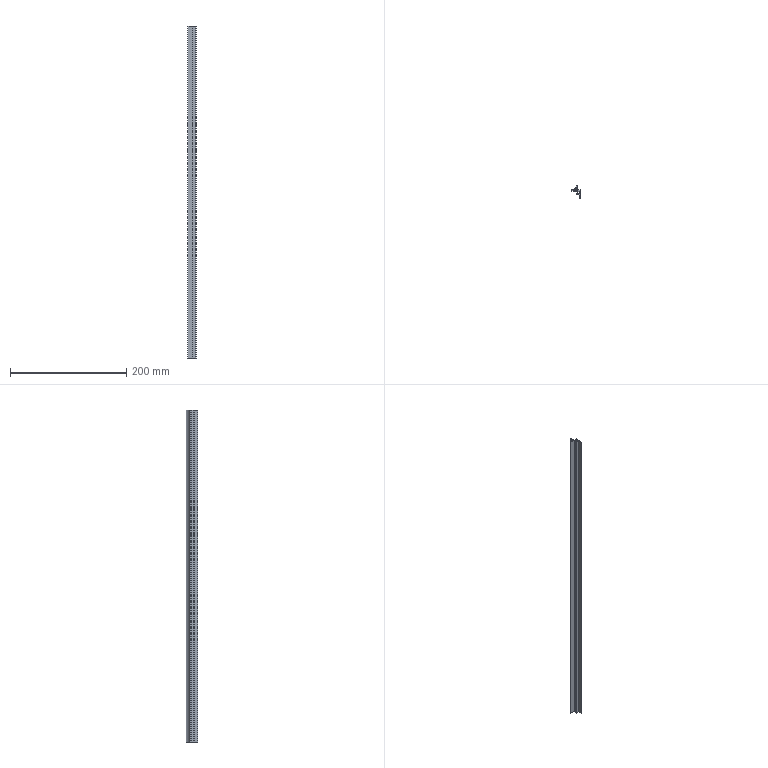Part | SolidWorks | features MoveFace 2, BaseBody 1, ICE 1 | 1 solid | 27 faces | box 14 x 20.3 x 571 mm | volume 29073 mm3 | plane 20 | cylinder 7 | commonest cylinder face diameters 0.387 x2 0.8 x2 0.4 x1 20 x1 22 x1
STEP:
#1=CARTESIAN_POINT('',(-5.304,-0.625,-587.));
#2=VERTEX_POINT('',#1);
#3=CARTESIAN_POINT('',(-5.449,-0.8125,-587.));
#4=VERTEX_POINT('',#3);
#5=CARTESIAN_POINT('',(-5.255,-0.8125,-587.));
#6=DIRECTION('',(0.,0.,1.));
#7=DIRECTION('',(-1.,0.,0.));
#8=AXIS2_PLACEMENT_3D('',#5,#6,#7);
#9=CIRCLE('',#8,0.1937);
#10=EDGE_CURVE('',#2,#4,#9,.T.);
#11=ORIENTED_EDGE('',*,*,#10,.T.);
#12=CARTESIAN_POINT('',(-5.449,-0.8125,-1158.));
#13=VERTEX_POINT('',#12);
#14=CARTESIAN_POINT('',(-5.449,-0.8125,230.));
#15=DIRECTION('',(0.,0.,-1.));
#16=VECTOR('',#15,1000.);
#17=LINE('',#14,#16);
#18=EDGE_CURVE('',#4,#13,#17,.T.);
#19=ORIENTED_EDGE('',*,*,#18,.T.);
#20=CARTESIAN_POINT('',(-5.304,-0.625,-1158.));
#21=VERTEX_POINT('',#20);
#22=CARTESIAN_POINT('',(-5.255,-0.8125,-1158.));
#23=DIRECTION('',(0.,0.,-1.));
#24=DIRECTION('',(1.,0.,0.));
#25=AXIS2_PLACEMENT_3D('',#22,#23,#24);
#26=CIRCLE('',#25,0.1937);
#27=EDGE_CURVE('',#13,#21,#26,.T.);
#28=ORIENTED_EDGE('',*,*,#27,.T.);
#29=CARTESIAN_POINT('',(-5.304,-0.625,230.));
#30=DIRECTION('',(0.,0.,-1.));
#31=VECTOR('',#30,1000.);
#32=LINE('',#29,#31);
#33=EDGE_CURVE('',#2,#21,#32,.T.);
#34=ORIENTED_EDGE('',*,*,#33,.F.);
#35=EDGE_LOOP('',(#11,#19,#28,#34));
#36=FACE_OUTER_BOUND('',#35,.T.);
#37=CARTESIAN_POINT('',(-5.255,-0.8125,230.));
#38=DIRECTION('',(0.,0.,-1.));
#39=DIRECTION('',(-1.,0.,0.));
#40=AXIS2_PLACEMENT_3D('',#37,#38,#39);
#41=CYLINDRICAL_SURFACE('',#40,0.1937);
#42=ADVANCED_FACE('',(#36),#41,.F.);
#43=CARTESIAN_POINT('',(5.,-1.,-1158.));
#44=VERTEX_POINT('',#43);
#45=CARTESIAN_POINT('',(5.,-14.3,-1158.));
#46=VERTEX_POINT('',#45);
#47=CARTESIAN_POINT('',(5.,29.623,-1158.));
#48=DIRECTION('',(0.,-1.,0.));
#49=VECTOR('',#48,1000.);
#50=LINE('',#47,#49);
#51=EDGE_CURVE('',#44,#46,#50,.T.);
#52=ORIENTED_EDGE('',*,*,#51,.F.);
#53=CARTESIAN_POINT('',(5.,-1.,-587.));
#54=VERTEX_POINT('',#53);
#55=CARTESIAN_POINT('',(5.,-1.,230.));
#56=DIRECTION('',(0.,0.,-1.));
#57=VECTOR('',#56,1000.);
#58=LINE('',#55,#57);
#59=EDGE_CURVE('',#54,#44,#58,.T.);
#60=ORIENTED_EDGE('',*,*,#59,.F.);
#61=CARTESIAN_POINT('',(5.,-14.3,-587.));
#62=VERTEX_POINT('',#61);
#63=CARTESIAN_POINT('',(5.,29.623,-587.));
#64=DIRECTION('',(0.,1.,0.));
#65=VECTOR('',#64,1000.);
#66=LINE('',#63,#65);
#67=EDGE_CURVE('',#62,#54,#66,.T.);
#68=ORIENTED_EDGE('',*,*,#67,.F.);
#69=CARTESIAN_POINT('',(5.,-14.3,230.));
#70=DIRECTION('',(0.,0.,1.));
#71=VECTOR('',#70,1000.);
#72=LINE('',#69,#71);
#73=EDGE_CURVE('',#46,#62,#72,.T.);
#74=ORIENTED_EDGE('',*,*,#73,.F.);
#75=EDGE_LOOP('',(#52,#60,#68,#74));
#76=FACE_OUTER_BOUND('',#75,.T.);
#77=CARTESIAN_POINT('',(5.,-14.3,230.));
#78=DIRECTION('',(-1.,0.,0.));
#79=DIRECTION('',(0.,0.,1.));
#80=AXIS2_PLACEMENT_3D('',#77,#78,#79);
#81=PLANE('',#80);
#82=ADVANCED_FACE('',(#76),#81,.F.);
#83=CARTESIAN_POINT('',(-9.,-2.,-1158.));
#84=VERTEX_POINT('',#83);
#85=CARTESIAN_POINT('',(-9.,-2.,-587.));
#86=VERTEX_POINT('',#85);
#87=CARTESIAN_POINT('',(-9.,-2.,230.));
#88=DIRECTION('',(0.,0.,1.));
#89=VECTOR('',#88,1000.);
#90=LINE('',#87,#89);
#91=EDGE_CURVE('',#84,#86,#90,.T.);
#92=ORIENTED_EDGE('',*,*,#91,.F.);
#93=CARTESIAN_POINT('',(0.9,-2.,-1158.));
#94=VERTEX_POINT('',#93);
#95=CARTESIAN_POINT('',(5.,-2.,-1158.));
#96=DIRECTION('',(-1.,0.,0.));
#97=VECTOR('',#96,1000.);
#98=LINE('',#95,#97);
#99=EDGE_CURVE('',#94,#84,#98,.T.);
#100=ORIENTED_EDGE('',*,*,#99,.F.);
#101=CARTESIAN_POINT('',(0.9,-2.,-587.));
#102=VERTEX_POINT('',#101);
#103=CARTESIAN_POINT('',(0.9,-2.,230.));
#104=DIRECTION('',(0.,0.,-1.));
#105=VECTOR('',#104,1000.);
#106=LINE('',#103,#105);
#107=EDGE_CURVE('',#102,#94,#106,.T.);
#108=ORIENTED_EDGE('',*,*,#107,.F.);
#109=CARTESIAN_POINT('',(5.,-2.,-587.));
#110=DIRECTION('',(1.,0.,0.));
#111=VECTOR('',#110,1000.);
#112=LINE('',#109,#111);
#113=EDGE_CURVE('',#86,#102,#112,.T.);
#114=ORIENTED_EDGE('',*,*,#113,.F.);
#115=EDGE_LOOP('',(#92,#100,#108,#114));
#116=FACE_OUTER_BOUND('',#115,.T.);
#117=CARTESIAN_POINT('',(-9.,-2.,230.));
#118=DIRECTION('',(0.,1.,0.));
#119=DIRECTION('',(0.,0.,1.));
#120=AXIS2_PLACEMENT_3D('',#117,#118,#119);
#121=PLANE('',#120);
#122=ADVANCED_FACE('',(#116),#121,.F.);
#123=CARTESIAN_POINT('',(4.,-6.,-587.));
#124=VERTEX_POINT('',#123);
#125=CARTESIAN_POINT('',(4.,-3.,-587.));
#126=VERTEX_POINT('',#125);
#127=CARTESIAN_POINT('',(4.,-3.,-587.));
#128=DIRECTION('',(0.,1.,0.));
#129=VECTOR('',#128,1000.);
#130=LINE('',#127,#129);
#131=EDGE_CURVE('',#124,#126,#130,.T.);
#132=ORIENTED_EDGE('',*,*,#131,.F.);
#133=CARTESIAN_POINT('',(1.,-6.,-587.));
#134=VERTEX_POINT('',#133);
#135=CARTESIAN_POINT('',(4.,-6.,-587.));
#136=DIRECTION('',(1.,0.,0.));
#137=VECTOR('',#136,1000.);
#138=LINE('',#135,#137);
#139=EDGE_CURVE('',#134,#124,#138,.T.);
#140=ORIENTED_EDGE('',*,*,#139,.F.);
#141=CARTESIAN_POINT('',(1.,-6.7,-587.));
#142=VERTEX_POINT('',#141);
#143=CARTESIAN_POINT('',(1.,29.623,-587.));
#144=DIRECTION('',(0.,-1.,0.));
#145=VECTOR('',#144,1000.);
#146=LINE('',#143,#145);
#147=EDGE_CURVE('',#134,#142,#146,.T.);
#148=ORIENTED_EDGE('',*,*,#147,.T.);
#149=CARTESIAN_POINT('',(-1.7,-6.7,-587.));
#150=VERTEX_POINT('',#149);
#151=CARTESIAN_POINT('',(1.,-6.7,-587.));
#152=DIRECTION('',(1.,0.,0.));
#153=VECTOR('',#152,1000.);
#154=LINE('',#151,#153);
#155=EDGE_CURVE('',#150,#142,#154,.T.);
#156=ORIENTED_EDGE('',*,*,#155,.F.);
#157=CARTESIAN_POINT('',(-1.7,-7.7,-587.));
#158=VERTEX_POINT('',#157);
#159=CARTESIAN_POINT('',(-1.7,29.623,-587.));
#160=DIRECTION('',(0.,-1.,0.));
#161=VECTOR('',#160,1000.);
#162=LINE('',#159,#161);
#163=EDGE_CURVE('',#150,#158,#162,.T.);
#164=ORIENTED_EDGE('',*,*,#163,.T.);
#165=CARTESIAN_POINT('',(4.,-7.7,-587.));
#166=VERTEX_POINT('',#165);
#167=CARTESIAN_POINT('',(-1.7,-7.7,-587.));
#168=DIRECTION('',(-1.,0.,0.));
#169=VECTOR('',#168,1000.);
#170=LINE('',#167,#169);
#171=EDGE_CURVE('',#166,#158,#170,.T.);
#172=ORIENTED_EDGE('',*,*,#171,.F.);
#173=CARTESIAN_POINT('',(4.,-14.3,-587.));
#174=VERTEX_POINT('',#173);
#175=CARTESIAN_POINT('',(4.,-7.7,-587.));
#176=DIRECTION('',(0.,1.,0.));
#177=VECTOR('',#176,1000.);
#178=LINE('',#175,#177);
#179=EDGE_CURVE('',#174,#166,#178,.T.);
#180=ORIENTED_EDGE('',*,*,#179,.F.);
#181=CARTESIAN_POINT('',(4.,-14.3,-587.));
#182=DIRECTION('',(-1.,0.,0.));
#183=VECTOR('',#182,1000.);
#184=LINE('',#181,#183);
#185=EDGE_CURVE('',#62,#174,#184,.T.);
#186=ORIENTED_EDGE('',*,*,#185,.F.);
#187=ORIENTED_EDGE('',*,*,#67,.T.);
#188=CARTESIAN_POINT('',(-5.207,-1.,-587.));
#189=VERTEX_POINT('',#188);
#190=CARTESIAN_POINT('',(5.,-1.,-587.));
#191=DIRECTION('',(1.,0.,0.));
#192=VECTOR('',#191,1000.);
#193=LINE('',#190,#192);
#194=EDGE_CURVE('',#189,#54,#193,.T.);
#195=ORIENTED_EDGE('',*,*,#194,.F.);
#196=CARTESIAN_POINT('',(-5.255,-0.8125,-587.));
#197=DIRECTION('',(0.,0.,1.));
#198=DIRECTION('',(-1.,0.,0.));
#199=AXIS2_PLACEMENT_3D('',#196,#197,#198);
#200=CIRCLE('',#199,0.1937);
#201=EDGE_CURVE('',#4,#189,#200,.T.);
#202=ORIENTED_EDGE('',*,*,#201,.F.);
#203=ORIENTED_EDGE('',*,*,#10,.F.);
#204=CARTESIAN_POINT('',(-1.368,3.063,-587.));
#205=VERTEX_POINT('',#204);
#206=CARTESIAN_POINT('',(-10.628,9.,-587.));
#207=DIRECTION('',(0.,0.,1.));
#208=DIRECTION('',(-1.,0.,0.));
#209=AXIS2_PLACEMENT_3D('',#206,#207,#208);
#210=CIRCLE('',#209,11.);
#211=EDGE_CURVE('',#2,#205,#210,.T.);
#212=ORIENTED_EDGE('',*,*,#211,.T.);
#213=CARTESIAN_POINT('',(-1.,2.955,-587.));
#214=VERTEX_POINT('',#213);
#215=CARTESIAN_POINT('',(-1.2,2.955,-587.));
#216=DIRECTION('',(0.,0.,1.));
#217=DIRECTION('',(-1.,0.,0.));
#218=AXIS2_PLACEMENT_3D('',#215,#216,#217);
#219=CIRCLE('',#218,0.2);
#220=EDGE_CURVE('',#214,#205,#219,.T.);
#221=ORIENTED_EDGE('',*,*,#220,.F.);
#222=CARTESIAN_POINT('',(-1.,1.5,-587.));
#223=VERTEX_POINT('',#222);
#224=CARTESIAN_POINT('',(-1.,2.955,-587.));
#225=DIRECTION('',(0.,1.,0.));
#226=VECTOR('',#225,1000.);
#227=LINE('',#224,#226);
#228=EDGE_CURVE('',#223,#214,#227,.T.);
#229=ORIENTED_EDGE('',*,*,#228,.F.);
#230=CARTESIAN_POINT('',(0.,1.5,-587.));
#231=VERTEX_POINT('',#230);
#232=CARTESIAN_POINT('',(-1.,1.5,-587.));
#233=DIRECTION('',(-1.,0.,0.));
#234=VECTOR('',#233,1000.);
#235=LINE('',#232,#234);
#236=EDGE_CURVE('',#231,#223,#235,.T.);
#237=ORIENTED_EDGE('',*,*,#236,.F.);
#238=CARTESIAN_POINT('',(0.,6.,-587.));
#239=VERTEX_POINT('',#238);
#240=CARTESIAN_POINT('',(0.,1.5,-587.));
#241=DIRECTION('',(0.,-1.,0.));
#242=VECTOR('',#241,1000.);
#243=LINE('',#240,#242);
#244=EDGE_CURVE('',#239,#231,#243,.T.);
#245=ORIENTED_EDGE('',*,*,#244,.F.);
#246=CARTESIAN_POINT('',(-0.8,6.,-587.));
#247=VERTEX_POINT('',#246);
#248=CARTESIAN_POINT('',(0.,6.,-587.));
#249=DIRECTION('',(1.,0.,0.));
#250=VECTOR('',#249,1000.);
#251=LINE('',#248,#250);
#252=EDGE_CURVE('',#247,#239,#251,.T.);
#253=ORIENTED_EDGE('',*,*,#252,.F.);
#254=CARTESIAN_POINT('',(-1.178,5.731,-587.));
#255=VERTEX_POINT('',#254);
#256=CARTESIAN_POINT('',(-0.8,5.6,-587.));
#257=DIRECTION('',(0.,0.,1.));
#258=DIRECTION('',(-1.,0.,0.));
#259=AXIS2_PLACEMENT_3D('',#256,#257,#258);
#260=CIRCLE('',#259,0.4);
#261=EDGE_CURVE('',#247,#255,#260,.T.);
#262=ORIENTED_EDGE('',*,*,#261,.T.);
#263=CARTESIAN_POINT('',(-8.678,-0.8077,-587.));
#264=VERTEX_POINT('',#263);
#265=CARTESIAN_POINT('',(-10.628,9.,-587.));
#266=DIRECTION('',(0.,0.,1.));
#267=DIRECTION('',(-1.,0.,0.));
#268=AXIS2_PLACEMENT_3D('',#265,#266,#267);
#269=CIRCLE('',#268,10.);
#270=EDGE_CURVE('',#264,#255,#269,.T.);
#271=ORIENTED_EDGE('',*,*,#270,.F.);
#272=CARTESIAN_POINT('',(-9.,-1.2,-587.));
#273=VERTEX_POINT('',#272);
#274=CARTESIAN_POINT('',(-8.6,-1.2,-587.));
#275=DIRECTION('',(0.,0.,1.));
#276=DIRECTION('',(-1.,0.,0.));
#277=AXIS2_PLACEMENT_3D('',#274,#275,#276);
#278=CIRCLE('',#277,0.4);
#279=EDGE_CURVE('',#264,#273,#278,.T.);
#280=ORIENTED_EDGE('',*,*,#279,.T.);
#281=CARTESIAN_POINT('',(-9.,29.623,-587.));
#282=DIRECTION('',(0.,-1.,0.));
#283=VECTOR('',#282,1000.);
#284=LINE('',#281,#283);
#285=EDGE_CURVE('',#273,#86,#284,.T.);
#286=ORIENTED_EDGE('',*,*,#285,.T.);
#287=ORIENTED_EDGE('',*,*,#113,.T.);
#288=CARTESIAN_POINT('',(0.9,-3.,-587.));
#289=VERTEX_POINT('',#288);
#290=CARTESIAN_POINT('',(0.9,-2.,-587.));
#291=DIRECTION('',(0.,1.,0.));
#292=VECTOR('',#291,1000.);
#293=LINE('',#290,#292);
#294=EDGE_CURVE('',#289,#102,#293,.T.);
#295=ORIENTED_EDGE('',*,*,#294,.F.);
#296=CARTESIAN_POINT('',(0.9,-3.,-587.));
#297=DIRECTION('',(-1.,0.,0.));
#298=VECTOR('',#297,1000.);
#299=LINE('',#296,#298);
#300=EDGE_CURVE('',#126,#289,#299,.T.);
#301=ORIENTED_EDGE('',*,*,#300,.F.);
#302=EDGE_LOOP('',(#132,#140,#148,#156,#164,#172,#180,#186,#187,#195,#202,#203,#212,#221,#229,#237,#245,#253,#262,#271,#280,#286,#287,#295,#301));
#303=FACE_OUTER_BOUND('',#302,.T.);
#304=CARTESIAN_POINT('',(5.,29.623,-587.));
#305=DIRECTION('',(0.,0.,-1.));
#306=DIRECTION('',(-1.,0.,0.));
#307=AXIS2_PLACEMENT_3D('',#304,#305,#306);
#308=PLANE('',#307);
#309=ADVANCED_FACE('',(#303),#308,.F.);
#310=ORIENTED_EDGE('',*,*,#185,.T.);
#311=CARTESIAN_POINT('',(4.,-14.3,-1158.));
#312=VERTEX_POINT('',#311);
#313=CARTESIAN_POINT('',(4.,-14.3,230.));
#314=DIRECTION('',(0.,0.,1.));
#315=VECTOR('',#314,1000.);
#316=LINE('',#313,#315);
#317=EDGE_CURVE('',#312,#174,#316,.T.);
#318=ORIENTED_EDGE('',*,*,#317,.F.);
#319=CARTESIAN_POINT('',(5.,-14.3,-1158.));
#320=DIRECTION('',(-1.,0.,0.));
#321=VECTOR('',#320,1000.);
#322=LINE('',#319,#321);
#323=EDGE_CURVE('',#46,#312,#322,.T.);
#324=ORIENTED_EDGE('',*,*,#323,.F.);
#325=ORIENTED_EDGE('',*,*,#73,.T.);
#326=EDGE_LOOP('',(#310,#318,#324,#325));
#327=FACE_OUTER_BOUND('',#326,.T.);
#328=CARTESIAN_POINT('',(4.,-14.3,230.));
#329=DIRECTION('',(0.,1.,0.));
#330=DIRECTION('',(0.,0.,1.));
#331=AXIS2_PLACEMENT_3D('',#328,#329,#330);
#332=PLANE('',#331);
#333=ADVANCED_FACE('',(#327),#332,.F.);
#334=ORIENTED_EDGE('',*,*,#51,.T.);
#335=ORIENTED_EDGE('',*,*,#323,.T.);
#336=CARTESIAN_POINT('',(4.,-7.7,-1158.));
#337=VERTEX_POINT('',#336);
#338=CARTESIAN_POINT('',(4.,-7.7,-1158.));
#339=DIRECTION('',(0.,-1.,0.));
#340=VECTOR('',#339,1000.);
#341=LINE('',#338,#340);
#342=EDGE_CURVE('',#337,#312,#341,.T.);
#343=ORIENTED_EDGE('',*,*,#342,.F.);
#344=CARTESIAN_POINT('',(-1.7,-7.7,-1158.));
#345=VERTEX_POINT('',#344);
#346=CARTESIAN_POINT('',(-1.7,-7.7,-1158.));
#347=DIRECTION('',(1.,0.,0.));
#348=VECTOR('',#347,1000.);
#349=LINE('',#346,#348);
#350=EDGE_CURVE('',#345,#337,#349,.T.);
#351=ORIENTED_EDGE('',*,*,#350,.F.);
#352=CARTESIAN_POINT('',(-1.7,-6.7,-1158.));
#353=VERTEX_POINT('',#352);
#354=CARTESIAN_POINT('',(-1.7,29.623,-1158.));
#355=DIRECTION('',(0.,1.,0.));
#356=VECTOR('',#355,1000.);
#357=LINE('',#354,#356);
#358=EDGE_CURVE('',#345,#353,#357,.T.);
#359=ORIENTED_EDGE('',*,*,#358,.T.);
#360=CARTESIAN_POINT('',(1.,-6.7,-1158.));
#361=VERTEX_POINT('',#360);
#362=CARTESIAN_POINT('',(1.,-6.7,-1158.));
#363=DIRECTION('',(-1.,0.,0.));
#364=VECTOR('',#363,1000.);
#365=LINE('',#362,#364);
#366=EDGE_CURVE('',#361,#353,#365,.T.);
#367=ORIENTED_EDGE('',*,*,#366,.F.);
#368=CARTESIAN_POINT('',(1.,-6.,-1158.));
#369=VERTEX_POINT('',#368);
#370=CARTESIAN_POINT('',(1.,29.623,-1158.));
#371=DIRECTION('',(0.,1.,0.));
#372=VECTOR('',#371,1000.);
#373=LINE('',#370,#372);
#374=EDGE_CURVE('',#361,#369,#373,.T.);
#375=ORIENTED_EDGE('',*,*,#374,.T.);
#376=CARTESIAN_POINT('',(4.,-6.,-1158.));
#377=VERTEX_POINT('',#376);
#378=CARTESIAN_POINT('',(4.,-6.,-1158.));
#379=DIRECTION('',(-1.,0.,0.));
#380=VECTOR('',#379,1000.);
#381=LINE('',#378,#380);
#382=EDGE_CURVE('',#377,#369,#381,.T.);
#383=ORIENTED_EDGE('',*,*,#382,.F.);
#384=CARTESIAN_POINT('',(4.,-3.,-1158.));
#385=VERTEX_POINT('',#384);
#386=CARTESIAN_POINT('',(4.,-3.,-1158.));
#387=DIRECTION('',(0.,-1.,0.));
#388=VECTOR('',#387,1000.);
#389=LINE('',#386,#388);
#390=EDGE_CURVE('',#385,#377,#389,.T.);
#391=ORIENTED_EDGE('',*,*,#390,.F.);
#392=CARTESIAN_POINT('',(0.9,-3.,-1158.));
#393=VERTEX_POINT('',#392);
#394=CARTESIAN_POINT('',(0.9,-3.,-1158.));
#395=DIRECTION('',(1.,0.,0.));
#396=VECTOR('',#395,1000.);
#397=LINE('',#394,#396);
#398=EDGE_CURVE('',#393,#385,#397,.T.);
#399=ORIENTED_EDGE('',*,*,#398,.F.);
#400=CARTESIAN_POINT('',(0.9,-2.,-1158.));
#401=DIRECTION('',(0.,-1.,0.));
#402=VECTOR('',#401,1000.);
#403=LINE('',#400,#402);
#404=EDGE_CURVE('',#94,#393,#403,.T.);
#405=ORIENTED_EDGE('',*,*,#404,.F.);
#406=ORIENTED_EDGE('',*,*,#99,.T.);
#407=CARTESIAN_POINT('',(-9.,-1.2,-1158.));
#408=VERTEX_POINT('',#407);
#409=CARTESIAN_POINT('',(-9.,-1.2,-1158.));
#410=DIRECTION('',(0.,-1.,0.));
#411=VECTOR('',#410,1000.);
#412=LINE('',#409,#411);
#413=EDGE_CURVE('',#408,#84,#412,.T.);
#414=ORIENTED_EDGE('',*,*,#413,.F.);
#415=CARTESIAN_POINT('',(-8.678,-0.8077,-1158.));
#416=VERTEX_POINT('',#415);
#417=CARTESIAN_POINT('',(-8.6,-1.2,-1158.));
#418=DIRECTION('',(0.,0.,-1.));
#419=DIRECTION('',(1.,0.,0.));
#420=AXIS2_PLACEMENT_3D('',#417,#418,#419);
#421=CIRCLE('',#420,0.4);
#422=EDGE_CURVE('',#408,#416,#421,.T.);
#423=ORIENTED_EDGE('',*,*,#422,.T.);
#424=CARTESIAN_POINT('',(-1.178,5.731,-1158.));
#425=VERTEX_POINT('',#424);
#426=CARTESIAN_POINT('',(-10.628,9.,-1158.));
#427=DIRECTION('',(0.,0.,-1.));
#428=DIRECTION('',(1.,0.,0.));
#429=AXIS2_PLACEMENT_3D('',#426,#427,#428);
#430=CIRCLE('',#429,10.);
#431=EDGE_CURVE('',#425,#416,#430,.T.);
#432=ORIENTED_EDGE('',*,*,#431,.F.);
#433=CARTESIAN_POINT('',(-0.8,6.,-1158.));
#434=VERTEX_POINT('',#433);
#435=CARTESIAN_POINT('',(-0.8,5.6,-1158.));
#436=DIRECTION('',(0.,0.,-1.));
#437=DIRECTION('',(1.,0.,0.));
#438=AXIS2_PLACEMENT_3D('',#435,#436,#437);
#439=CIRCLE('',#438,0.4);
#440=EDGE_CURVE('',#425,#434,#439,.T.);
#441=ORIENTED_EDGE('',*,*,#440,.T.);
#442=CARTESIAN_POINT('',(0.,6.,-1158.));
#443=VERTEX_POINT('',#442);
#444=CARTESIAN_POINT('',(0.,6.,-1158.));
#445=DIRECTION('',(-1.,0.,0.));
#446=VECTOR('',#445,1000.);
#447=LINE('',#444,#446);
#448=EDGE_CURVE('',#443,#434,#447,.T.);
#449=ORIENTED_EDGE('',*,*,#448,.F.);
#450=CARTESIAN_POINT('',(0.,1.5,-1158.));
#451=VERTEX_POINT('',#450);
#452=CARTESIAN_POINT('',(0.,1.5,-1158.));
#453=DIRECTION('',(0.,1.,0.));
#454=VECTOR('',#453,1000.);
#455=LINE('',#452,#454);
#456=EDGE_CURVE('',#451,#443,#455,.T.);
#457=ORIENTED_EDGE('',*,*,#456,.F.);
#458=CARTESIAN_POINT('',(-1.,1.5,-1158.));
#459=VERTEX_POINT('',#458);
#460=CARTESIAN_POINT('',(-1.,1.5,-1158.));
#461=DIRECTION('',(1.,0.,0.));
#462=VECTOR('',#461,1000.);
#463=LINE('',#460,#462);
#464=EDGE_CURVE('',#459,#451,#463,.T.);
#465=ORIENTED_EDGE('',*,*,#464,.F.);
#466=CARTESIAN_POINT('',(-1.,2.955,-1158.));
#467=VERTEX_POINT('',#466);
#468=CARTESIAN_POINT('',(-1.,2.955,-1158.));
#469=DIRECTION('',(0.,-1.,0.));
#470=VECTOR('',#469,1000.);
#471=LINE('',#468,#470);
#472=EDGE_CURVE('',#467,#459,#471,.T.);
#473=ORIENTED_EDGE('',*,*,#472,.F.);
#474=CARTESIAN_POINT('',(-1.368,3.063,-1158.));
#475=VERTEX_POINT('',#474);
#476=CARTESIAN_POINT('',(-1.2,2.955,-1158.));
#477=DIRECTION('',(0.,0.,-1.));
#478=DIRECTION('',(1.,0.,0.));
#479=AXIS2_PLACEMENT_3D('',#476,#477,#478);
#480=CIRCLE('',#479,0.2);
#481=EDGE_CURVE('',#475,#467,#480,.T.);
#482=ORIENTED_EDGE('',*,*,#481,.F.);
#483=CARTESIAN_POINT('',(-10.628,9.,-1158.));
#484=DIRECTION('',(0.,0.,-1.));
#485=DIRECTION('',(1.,0.,0.));
#486=AXIS2_PLACEMENT_3D('',#483,#484,#485);
#487=CIRCLE('',#486,11.);
#488=EDGE_CURVE('',#475,#21,#487,.T.);
#489=ORIENTED_EDGE('',*,*,#488,.T.);
#490=ORIENTED_EDGE('',*,*,#27,.F.);
#491=CARTESIAN_POINT('',(-5.207,-1.,-1158.));
#492=VERTEX_POINT('',#491);
#493=CARTESIAN_POINT('',(-5.255,-0.8125,-1158.));
#494=DIRECTION('',(0.,0.,-1.));
#495=DIRECTION('',(1.,0.,0.));
#496=AXIS2_PLACEMENT_3D('',#493,#494,#495);
#497=CIRCLE('',#496,0.1937);
#498=EDGE_CURVE('',#492,#13,#497,.T.);
#499=ORIENTED_EDGE('',*,*,#498,.F.);
#500=CARTESIAN_POINT('',(5.,-1.,-1158.));
#501=DIRECTION('',(-1.,0.,0.));
#502=VECTOR('',#501,1000.);
#503=LINE('',#500,#502);
#504=EDGE_CURVE('',#44,#492,#503,.T.);
#505=ORIENTED_EDGE('',*,*,#504,.F.);
#506=EDGE_LOOP('',(#334,#335,#343,#351,#359,#367,#375,#383,#391,#399,#405,#406,#414,#423,#432,#441,#449,#457,#465,#473,#482,#489,#490,#499,#505));
#507=FACE_OUTER_BOUND('',#506,.T.);
#508=CARTESIAN_POINT('',(5.,29.623,-1158.));
#509=DIRECTION('',(0.,0.,1.));
#510=DIRECTION('',(1.,0.,0.));
#511=AXIS2_PLACEMENT_3D('',#508,#509,#510);
#512=PLANE('',#511);
#513=ADVANCED_FACE('',(#507),#512,.F.);
#514=ORIENTED_EDGE('',*,*,#59,.T.);
#515=ORIENTED_EDGE('',*,*,#504,.T.);
#516=CARTESIAN_POINT('',(-5.207,-1.,230.));
#517=DIRECTION('',(0.,0.,-1.));
#518=VECTOR('',#517,1000.);
#519=LINE('',#516,#518);
#520=EDGE_CURVE('',#189,#492,#519,.T.);
#521=ORIENTED_EDGE('',*,*,#520,.F.);
#522=ORIENTED_EDGE('',*,*,#194,.T.);
#523=EDGE_LOOP('',(#514,#515,#521,#522));
#524=FACE_OUTER_BOUND('',#523,.T.);
#525=CARTESIAN_POINT('',(5.,-1.,230.));
#526=DIRECTION('',(0.,-1.,0.));
#527=DIRECTION('',(0.,0.,-1.));
#528=AXIS2_PLACEMENT_3D('',#525,#526,#527);
#529=PLANE('',#528);
#530=ADVANCED_FACE('',(#524),#529,.F.);
#531=CARTESIAN_POINT('',(-9.,-1.2,230.));
#532=DIRECTION('',(0.,0.,1.));
#533=VECTOR('',#532,1000.);
#534=LINE('',#531,#533);
#535=EDGE_CURVE('',#408,#273,#534,.T.);
#536=ORIENTED_EDGE('',*,*,#535,.F.);
#537=ORIENTED_EDGE('',*,*,#413,.T.);
#538=ORIENTED_EDGE('',*,*,#91,.T.);
#539=ORIENTED_EDGE('',*,*,#285,.F.);
#540=EDGE_LOOP('',(#536,#537,#538,#539));
#541=FACE_OUTER_BOUND('',#540,.T.);
#542=CARTESIAN_POINT('',(-9.,-1.2,230.));
#543=DIRECTION('',(1.,0.,0.));
#544=DIRECTION('',(0.,0.,-1.));
#545=AXIS2_PLACEMENT_3D('',#542,#543,#544);
#546=PLANE('',#545);
#547=ADVANCED_FACE('',(#541),#546,.F.);
#548=ORIENTED_EDGE('',*,*,#294,.T.);
#549=ORIENTED_EDGE('',*,*,#107,.T.);
#550=ORIENTED_EDGE('',*,*,#404,.T.);
#551=CARTESIAN_POINT('',(0.9,-3.,230.));
#552=DIRECTION('',(0.,0.,-1.));
#553=VECTOR('',#552,1000.);
#554=LINE('',#551,#553);
#555=EDGE_CURVE('',#289,#393,#554,.T.);
#556=ORIENTED_EDGE('',*,*,#555,.F.);
#557=EDGE_LOOP('',(#548,#549,#550,#556));
#558=FACE_OUTER_BOUND('',#557,.T.);
#559=CARTESIAN_POINT('',(0.9,-2.,230.));
#560=DIRECTION('',(1.,0.,0.));
#561=DIRECTION('',(0.,0.,-1.));
#562=AXIS2_PLACEMENT_3D('',#559,#560,#561);
#563=PLANE('',#562);
#564=ADVANCED_FACE('',(#558),#563,.F.);
#565=ORIENTED_EDGE('',*,*,#300,.T.);
#566=ORIENTED_EDGE('',*,*,#555,.T.);
#567=ORIENTED_EDGE('',*,*,#398,.T.);
#568=CARTESIAN_POINT('',(4.,-3.,230.));
#569=DIRECTION('',(0.,0.,-1.));
#570=VECTOR('',#569,1000.);
#571=LINE('',#568,#570);
#572=EDGE_CURVE('',#126,#385,#571,.T.);
#573=ORIENTED_EDGE('',*,*,#572,.F.);
#574=EDGE_LOOP('',(#565,#566,#567,#573));
#575=FACE_OUTER_BOUND('',#574,.T.);
#576=CARTESIAN_POINT('',(0.9,-3.,230.));
#577=DIRECTION('',(0.,1.,0.));
#578=DIRECTION('',(0.,0.,1.));
#579=AXIS2_PLACEMENT_3D('',#576,#577,#578);
#580=PLANE('',#579);
#581=ADVANCED_FACE('',(#575),#580,.F.);
#582=ORIENTED_EDGE('',*,*,#131,.T.);
#583=ORIENTED_EDGE('',*,*,#572,.T.);
#584=ORIENTED_EDGE('',*,*,#390,.T.);
#585=CARTESIAN_POINT('',(4.,-6.,230.));
#586=DIRECTION('',(0.,0.,-1.));
#587=VECTOR('',#586,1000.);
#588=LINE('',#585,#587);
#589=EDGE_CURVE('',#124,#377,#588,.T.);
#590=ORIENTED_EDGE('',*,*,#589,.F.);
#591=EDGE_LOOP('',(#582,#583,#584,#590));
#592=FACE_OUTER_BOUND('',#591,.T.);
#593=CARTESIAN_POINT('',(4.,-3.,230.));
#594=DIRECTION('',(1.,0.,0.));
#595=DIRECTION('',(0.,0.,-1.));
#596=AXIS2_PLACEMENT_3D('',#593,#594,#595);
#597=PLANE('',#596);
#598=ADVANCED_FACE('',(#592),#597,.F.);
#599=ORIENTED_EDGE('',*,*,#139,.T.);
#600=ORIENTED_EDGE('',*,*,#589,.T.);
#601=ORIENTED_EDGE('',*,*,#382,.T.);
#602=CARTESIAN_POINT('',(1.,-6.,230.));
#603=DIRECTION('',(0.,0.,-1.));
#604=VECTOR('',#603,1000.);
#605=LINE('',#602,#604);
#606=EDGE_CURVE('',#134,#369,#605,.T.);
#607=ORIENTED_EDGE('',*,*,#606,.F.);
#608=EDGE_LOOP('',(#599,#600,#601,#607));
#609=FACE_OUTER_BOUND('',#608,.T.);
#610=CARTESIAN_POINT('',(4.,-6.,230.));
#611=DIRECTION('',(0.,-1.,0.));
#612=DIRECTION('',(0.,0.,-1.));
#613=AXIS2_PLACEMENT_3D('',#610,#611,#612);
#614=PLANE('',#613);
#615=ADVANCED_FACE('',(#609),#614,.F.);
#616=ORIENTED_EDGE('',*,*,#155,.T.);
#617=CARTESIAN_POINT('',(1.,-6.7,230.));
#618=DIRECTION('',(0.,0.,1.));
#619=VECTOR('',#618,1000.);
#620=LINE('',#617,#619);
#621=EDGE_CURVE('',#361,#142,#620,.T.);
#622=ORIENTED_EDGE('',*,*,#621,.F.);
#623=ORIENTED_EDGE('',*,*,#366,.T.);
#624=CARTESIAN_POINT('',(-1.7,-6.7,230.));
#625=DIRECTION('',(0.,0.,-1.));
#626=VECTOR('',#625,1000.);
#627=LINE('',#624,#626);
#628=EDGE_CURVE('',#150,#353,#627,.T.);
#629=ORIENTED_EDGE('',*,*,#628,.F.);
#630=EDGE_LOOP('',(#616,#622,#623,#629));
#631=FACE_OUTER_BOUND('',#630,.T.);
#632=CARTESIAN_POINT('',(1.,-6.7,230.));
#633=DIRECTION('',(0.,-1.,0.));
#634=DIRECTION('',(0.,0.,-1.));
#635=AXIS2_PLACEMENT_3D('',#632,#633,#634);
#636=PLANE('',#635);
#637=ADVANCED_FACE('',(#631),#636,.F.);
#638=ORIENTED_EDGE('',*,*,#171,.T.);
#639=CARTESIAN_POINT('',(-1.7,-7.7,230.));
#640=DIRECTION('',(0.,0.,1.));
#641=VECTOR('',#640,1000.);
#642=LINE('',#639,#641);
#643=EDGE_CURVE('',#345,#158,#642,.T.);
#644=ORIENTED_EDGE('',*,*,#643,.F.);
#645=ORIENTED_EDGE('',*,*,#350,.T.);
#646=CARTESIAN_POINT('',(4.,-7.7,230.));
#647=DIRECTION('',(0.,0.,-1.));
#648=VECTOR('',#647,1000.);
#649=LINE('',#646,#648);
#650=EDGE_CURVE('',#166,#337,#649,.T.);
#651=ORIENTED_EDGE('',*,*,#650,.F.);
#652=EDGE_LOOP('',(#638,#644,#645,#651));
#653=FACE_OUTER_BOUND('',#652,.T.);
#654=CARTESIAN_POINT('',(-1.7,-7.7,230.));
#655=DIRECTION('',(0.,1.,0.));
#656=DIRECTION('',(0.,0.,1.));
#657=AXIS2_PLACEMENT_3D('',#654,#655,#656);
#658=PLANE('',#657);
#659=ADVANCED_FACE('',(#653),#658,.F.);
#660=ORIENTED_EDGE('',*,*,#179,.T.);
#661=ORIENTED_EDGE('',*,*,#650,.T.);
#662=ORIENTED_EDGE('',*,*,#342,.T.);
#663=ORIENTED_EDGE('',*,*,#317,.T.);
#664=EDGE_LOOP('',(#660,#661,#662,#663));
#665=FACE_OUTER_BOUND('',#664,.T.);
#666=CARTESIAN_POINT('',(4.,-7.7,230.));
#667=DIRECTION('',(1.,0.,0.));
#668=DIRECTION('',(0.,0.,-1.));
#669=AXIS2_PLACEMENT_3D('',#666,#667,#668);
#670=PLANE('',#669);
#671=ADVANCED_FACE('',(#665),#670,.F.);
#672=ORIENTED_EDGE('',*,*,#18,.F.);
#673=ORIENTED_EDGE('',*,*,#201,.T.);
#674=ORIENTED_EDGE('',*,*,#520,.T.);
#675=ORIENTED_EDGE('',*,*,#498,.T.);
#676=EDGE_LOOP('',(#672,#673,#674,#675));
#677=FACE_OUTER_BOUND('',#676,.T.);
#678=CARTESIAN_POINT('',(-5.255,-0.8125,230.));
#679=DIRECTION('',(0.,0.,-1.));
#680=DIRECTION('',(-1.,0.,0.));
#681=AXIS2_PLACEMENT_3D('',#678,#679,#680);
#682=CYLINDRICAL_SURFACE('',#681,0.1937);
#683=ADVANCED_FACE('',(#677),#682,.F.);
#684=CARTESIAN_POINT('',(-1.,2.955,230.));
#685=DIRECTION('',(0.,0.,1.));
#686=VECTOR('',#685,1000.);
#687=LINE('',#684,#686);
#688=EDGE_CURVE('',#467,#214,#687,.T.);
#689=ORIENTED_EDGE('',*,*,#688,.F.);
#690=ORIENTED_EDGE('',*,*,#472,.T.);
#691=CARTESIAN_POINT('',(-1.,1.5,230.));
#692=DIRECTION('',(0.,0.,-1.));
#693=VECTOR('',#692,1000.);
#694=LINE('',#691,#693);
#695=EDGE_CURVE('',#223,#459,#694,.T.);
#696=ORIENTED_EDGE('',*,*,#695,.F.);
#697=ORIENTED_EDGE('',*,*,#228,.T.);
#698=EDGE_LOOP('',(#689,#690,#696,#697));
#699=FACE_OUTER_BOUND('',#698,.T.);
#700=CARTESIAN_POINT('',(-1.,2.955,230.));
#701=DIRECTION('',(1.,0.,0.));
#702=DIRECTION('',(0.,0.,-1.));
#703=AXIS2_PLACEMENT_3D('',#700,#701,#702);
#704=PLANE('',#703);
#705=ADVANCED_FACE('',(#699),#704,.F.);
#706=ORIENTED_EDGE('',*,*,#488,.F.);
#707=CARTESIAN_POINT('',(-1.368,3.063,230.));
#708=DIRECTION('',(0.,0.,1.));
#709=VECTOR('',#708,1000.);
#710=LINE('',#707,#709);
#711=EDGE_CURVE('',#475,#205,#710,.T.);
#712=ORIENTED_EDGE('',*,*,#711,.T.);
#713=ORIENTED_EDGE('',*,*,#211,.F.);
#714=ORIENTED_EDGE('',*,*,#33,.T.);
#715=EDGE_LOOP('',(#706,#712,#713,#714));
#716=FACE_OUTER_BOUND('',#715,.T.);
#717=CARTESIAN_POINT('',(-10.628,9.,230.));
#718=DIRECTION('',(0.,0.,-1.));
#719=DIRECTION('',(-1.,0.,0.));
#720=AXIS2_PLACEMENT_3D('',#717,#718,#719);
#721=CYLINDRICAL_SURFACE('',#720,11.);
#722=ADVANCED_FACE('',(#716),#721,.T.);
#723=CARTESIAN_POINT('',(-1.178,5.731,230.));
#724=DIRECTION('',(0.,0.,1.));
#725=VECTOR('',#724,1000.);
#726=LINE('',#723,#725);
#727=EDGE_CURVE('',#425,#255,#726,.T.);
#728=ORIENTED_EDGE('',*,*,#727,.F.);
#729=ORIENTED_EDGE('',*,*,#431,.T.);
#730=CARTESIAN_POINT('',(-8.678,-0.8077,230.));
#731=DIRECTION('',(0.,0.,-1.));
#732=VECTOR('',#731,1000.);
#733=LINE('',#730,#732);
#734=EDGE_CURVE('',#264,#416,#733,.T.);
#735=ORIENTED_EDGE('',*,*,#734,.F.);
#736=ORIENTED_EDGE('',*,*,#270,.T.);
#737=EDGE_LOOP('',(#728,#729,#735,#736));
#738=FACE_OUTER_BOUND('',#737,.T.);
#739=CARTESIAN_POINT('',(-10.628,9.,230.));
#740=DIRECTION('',(0.,0.,-1.));
#741=DIRECTION('',(-1.,0.,0.));
#742=AXIS2_PLACEMENT_3D('',#739,#740,#741);
#743=CYLINDRICAL_SURFACE('',#742,10.);
#744=ADVANCED_FACE('',(#738),#743,.F.);
#745=CARTESIAN_POINT('',(0.,1.5,230.));
#746=DIRECTION('',(0.,0.,1.));
#747=VECTOR('',#746,1000.);
#748=LINE('',#745,#747);
#749=EDGE_CURVE('',#451,#231,#748,.T.);
#750=ORIENTED_EDGE('',*,*,#749,.F.);
#751=ORIENTED_EDGE('',*,*,#456,.T.);
#752=CARTESIAN_POINT('',(0.,6.,230.));
#753=DIRECTION('',(0.,0.,-1.));
#754=VECTOR('',#753,1000.);
#755=LINE('',#752,#754);
#756=EDGE_CURVE('',#239,#443,#755,.T.);
#757=ORIENTED_EDGE('',*,*,#756,.F.);
#758=ORIENTED_EDGE('',*,*,#244,.T.);
#759=EDGE_LOOP('',(#750,#751,#757,#758));
#760=FACE_OUTER_BOUND('',#759,.T.);
#761=CARTESIAN_POINT('',(0.,1.5,230.));
#762=DIRECTION('',(-1.,0.,0.));
#763=DIRECTION('',(0.,0.,1.));
#764=AXIS2_PLACEMENT_3D('',#761,#762,#763);
#765=PLANE('',#764);
#766=ADVANCED_FACE('',(#760),#765,.F.);
#767=ORIENTED_EDGE('',*,*,#422,.F.);
#768=ORIENTED_EDGE('',*,*,#535,.T.);
#769=ORIENTED_EDGE('',*,*,#279,.F.);
#770=ORIENTED_EDGE('',*,*,#734,.T.);
#771=EDGE_LOOP('',(#767,#768,#769,#770));
#772=FACE_OUTER_BOUND('',#771,.T.);
#773=CARTESIAN_POINT('',(-8.6,-1.2,230.));
#774=DIRECTION('',(0.,0.,-1.));
#775=DIRECTION('',(-1.,0.,0.));
#776=AXIS2_PLACEMENT_3D('',#773,#774,#775);
#777=CYLINDRICAL_SURFACE('',#776,0.4);
#778=ADVANCED_FACE('',(#772),#777,.T.);
#779=ORIENTED_EDGE('',*,*,#147,.F.);
#780=ORIENTED_EDGE('',*,*,#606,.T.);
#781=ORIENTED_EDGE('',*,*,#374,.F.);
#782=ORIENTED_EDGE('',*,*,#621,.T.);
#783=EDGE_LOOP('',(#779,#780,#781,#782));
#784=FACE_OUTER_BOUND('',#783,.T.);
#785=CARTESIAN_POINT('',(1.,-6.,230.));
#786=DIRECTION('',(1.,0.,0.));
#787=DIRECTION('',(0.,0.,-1.));
#788=AXIS2_PLACEMENT_3D('',#785,#786,#787);
#789=PLANE('',#788);
#790=ADVANCED_FACE('',(#784),#789,.F.);
#791=ORIENTED_EDGE('',*,*,#163,.F.);
#792=ORIENTED_EDGE('',*,*,#628,.T.);
#793=ORIENTED_EDGE('',*,*,#358,.F.);
#794=ORIENTED_EDGE('',*,*,#643,.T.);
#795=EDGE_LOOP('',(#791,#792,#793,#794));
#796=FACE_OUTER_BOUND('',#795,.T.);
#797=CARTESIAN_POINT('',(-1.7,-6.7,230.));
#798=DIRECTION('',(1.,0.,0.));
#799=DIRECTION('',(0.,0.,-1.));
#800=AXIS2_PLACEMENT_3D('',#797,#798,#799);
#801=PLANE('',#800);
#802=ADVANCED_FACE('',(#796),#801,.F.);
#803=ORIENTED_EDGE('',*,*,#711,.F.);
#804=ORIENTED_EDGE('',*,*,#481,.T.);
#805=ORIENTED_EDGE('',*,*,#688,.T.);
#806=ORIENTED_EDGE('',*,*,#220,.T.);
#807=EDGE_LOOP('',(#803,#804,#805,#806));
#808=FACE_OUTER_BOUND('',#807,.T.);
#809=CARTESIAN_POINT('',(-1.2,2.955,230.));
#810=DIRECTION('',(0.,0.,-1.));
#811=DIRECTION('',(-1.,0.,0.));
#812=AXIS2_PLACEMENT_3D('',#809,#810,#811);
#813=CYLINDRICAL_SURFACE('',#812,0.2);
#814=ADVANCED_FACE('',(#808),#813,.F.);
#815=ORIENTED_EDGE('',*,*,#695,.T.);
#816=ORIENTED_EDGE('',*,*,#464,.T.);
#817=ORIENTED_EDGE('',*,*,#749,.T.);
#818=ORIENTED_EDGE('',*,*,#236,.T.);
#819=EDGE_LOOP('',(#815,#816,#817,#818));
#820=FACE_OUTER_BOUND('',#819,.T.);
#821=CARTESIAN_POINT('',(-1.,1.5,230.));
#822=DIRECTION('',(0.,1.,0.));
#823=DIRECTION('',(0.,0.,1.));
#824=AXIS2_PLACEMENT_3D('',#821,#822,#823);
#825=PLANE('',#824);
#826=ADVANCED_FACE('',(#820),#825,.F.);
#827=ORIENTED_EDGE('',*,*,#440,.F.);
#828=ORIENTED_EDGE('',*,*,#727,.T.);
#829=ORIENTED_EDGE('',*,*,#261,.F.);
#830=CARTESIAN_POINT('',(-0.8,6.,230.));
#831=DIRECTION('',(0.,0.,-1.));
#832=VECTOR('',#831,1000.);
#833=LINE('',#830,#832);
#834=EDGE_CURVE('',#247,#434,#833,.T.);
#835=ORIENTED_EDGE('',*,*,#834,.T.);
#836=EDGE_LOOP('',(#827,#828,#829,#835));
#837=FACE_OUTER_BOUND('',#836,.T.);
#838=CARTESIAN_POINT('',(-0.8,5.6,230.));
#839=DIRECTION('',(0.,0.,-1.));
#840=DIRECTION('',(-1.,0.,0.));
#841=AXIS2_PLACEMENT_3D('',#838,#839,#840);
#842=CYLINDRICAL_SURFACE('',#841,0.4);
#843=ADVANCED_FACE('',(#837),#842,.T.);
#844=ORIENTED_EDGE('',*,*,#756,.T.);
#845=ORIENTED_EDGE('',*,*,#448,.T.);
#846=ORIENTED_EDGE('',*,*,#834,.F.);
#847=ORIENTED_EDGE('',*,*,#252,.T.);
#848=EDGE_LOOP('',(#844,#845,#846,#847));
#849=FACE_OUTER_BOUND('',#848,.T.);
#850=CARTESIAN_POINT('',(0.,6.,230.));
#851=DIRECTION('',(0.,-1.,0.));
#852=DIRECTION('',(0.,0.,-1.));
#853=AXIS2_PLACEMENT_3D('',#850,#851,#852);
#854=PLANE('',#853);
#855=ADVANCED_FACE('',(#849),#854,.F.);
#856=CLOSED_SHELL('',(#42,#82,#122,#309,#333,#513,#530,#547,#564,#581,#598,#615,#637,#659,#671,#683,#705,#722,#744,#766,#778,#790,#802,#814,#826,#843,#855));
#857=MANIFOLD_SOLID_BREP('',#856);
#858=CARTESIAN_POINT('',(0.,0.,0.));
#859=DIRECTION('',(0.,0.,1.));
#860=DIRECTION('',(1.,0.,0.));
#861=AXIS2_PLACEMENT_3D('',#858,#859,#860);
#862=(LENGTH_UNIT()NAMED_UNIT(*)SI_UNIT(.MILLI.,.METRE.));
#863=UNCERTAINTY_MEASURE_WITH_UNIT(LENGTH_MEASURE(0.00001),#862,'','');
#864=(NAMED_UNIT(*)PLANE_ANGLE_UNIT()SI_UNIT($,.RADIAN.));
#865=(NAMED_UNIT(*)SI_UNIT($,.STERADIAN.)SOLID_ANGLE_UNIT());
#866=(GEOMETRIC_REPRESENTATION_CONTEXT(3)GLOBAL_UNCERTAINTY_ASSIGNED_CONTEXT((#863))GLOBAL_UNIT_ASSIGNED_CONTEXT((#862,#864,#865))REPRESENTATION_CONTEXT('',''));
#867=ADVANCED_BREP_SHAPE_REPRESENTATION('',(#857,#861),#866);